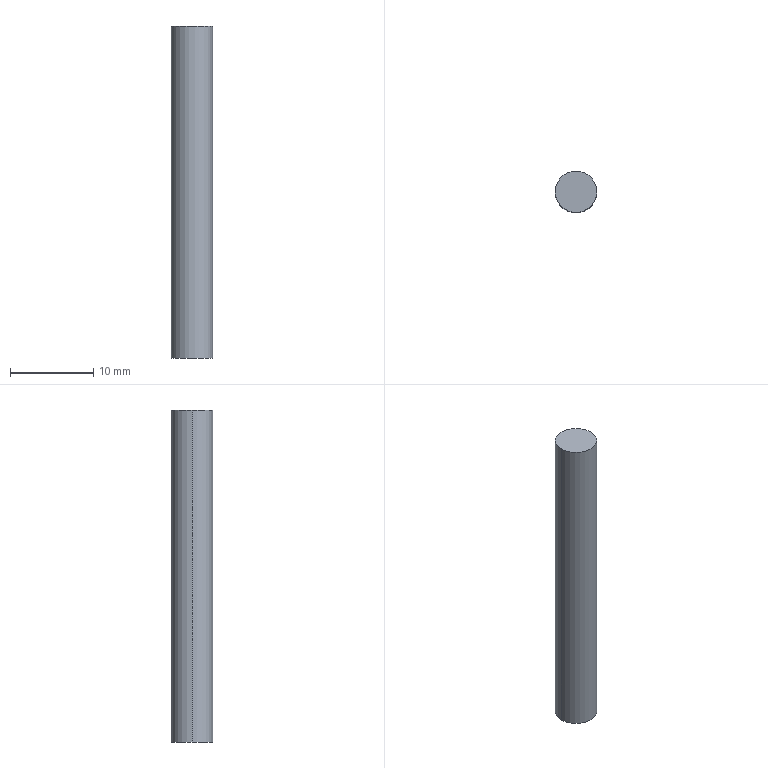Part | SolidWorks | features Extrusion 1 | 1 solid | 4 faces | box 5 x 5 x 40 mm | volume 785.398 mm3 | cylinder 2 | plane 2 | commonest cylinder face diameters 5 x2
STEP:
#1=CARTESIAN_POINT('',(2.5,0.,40.));
#2=VERTEX_POINT('',#1);
#3=CARTESIAN_POINT('',(-2.5,0.,40.));
#4=VERTEX_POINT('',#3);
#5=CARTESIAN_POINT('',(0.,0.,40.));
#6=DIRECTION('',(0.,0.,1.));
#7=DIRECTION('',(1.,0.,0.));
#8=AXIS2_PLACEMENT_3D('',#5,#6,#7);
#9=CIRCLE('',#8,2.5);
#10=EDGE_CURVE('',#2,#4,#9,.T.);
#11=ORIENTED_EDGE('',*,*,#10,.F.);
#12=CARTESIAN_POINT('',(2.5,0.,0.));
#13=VERTEX_POINT('',#12);
#14=CARTESIAN_POINT('',(2.5,0.,40.));
#15=DIRECTION('',(0.,0.,-1.));
#16=VECTOR('',#15,1000.);
#17=LINE('',#14,#16);
#18=EDGE_CURVE('',#2,#13,#17,.T.);
#19=ORIENTED_EDGE('',*,*,#18,.T.);
#20=CARTESIAN_POINT('',(-2.5,0.,0.));
#21=VERTEX_POINT('',#20);
#22=CARTESIAN_POINT('',(0.,0.,0.));
#23=DIRECTION('',(0.,0.,1.));
#24=DIRECTION('',(1.,0.,0.));
#25=AXIS2_PLACEMENT_3D('',#22,#23,#24);
#26=CIRCLE('',#25,2.5);
#27=EDGE_CURVE('',#13,#21,#26,.T.);
#28=ORIENTED_EDGE('',*,*,#27,.T.);
#29=CARTESIAN_POINT('',(-2.5,0.,40.));
#30=DIRECTION('',(0.,0.,-1.));
#31=VECTOR('',#30,1000.);
#32=LINE('',#29,#31);
#33=EDGE_CURVE('',#4,#21,#32,.T.);
#34=ORIENTED_EDGE('',*,*,#33,.F.);
#35=EDGE_LOOP('',(#11,#19,#28,#34));
#36=FACE_OUTER_BOUND('',#35,.T.);
#37=CARTESIAN_POINT('',(0.,0.,40.));
#38=DIRECTION('',(0.,0.,-1.));
#39=DIRECTION('',(-1.,0.,0.));
#40=AXIS2_PLACEMENT_3D('',#37,#38,#39);
#41=CYLINDRICAL_SURFACE('',#40,2.5);
#42=ADVANCED_FACE('',(#36),#41,.T.);
#43=ORIENTED_EDGE('',*,*,#18,.F.);
#44=CARTESIAN_POINT('',(0.,0.,40.));
#45=DIRECTION('',(0.,0.,1.));
#46=DIRECTION('',(1.,0.,0.));
#47=AXIS2_PLACEMENT_3D('',#44,#45,#46);
#48=CIRCLE('',#47,2.5);
#49=EDGE_CURVE('',#4,#2,#48,.T.);
#50=ORIENTED_EDGE('',*,*,#49,.F.);
#51=ORIENTED_EDGE('',*,*,#33,.T.);
#52=CARTESIAN_POINT('',(0.,0.,0.));
#53=DIRECTION('',(0.,0.,1.));
#54=DIRECTION('',(1.,0.,0.));
#55=AXIS2_PLACEMENT_3D('',#52,#53,#54);
#56=CIRCLE('',#55,2.5);
#57=EDGE_CURVE('',#21,#13,#56,.T.);
#58=ORIENTED_EDGE('',*,*,#57,.T.);
#59=EDGE_LOOP('',(#43,#50,#51,#58));
#60=FACE_OUTER_BOUND('',#59,.T.);
#61=CARTESIAN_POINT('',(0.,0.,40.));
#62=DIRECTION('',(0.,0.,-1.));
#63=DIRECTION('',(-1.,0.,0.));
#64=AXIS2_PLACEMENT_3D('',#61,#62,#63);
#65=CYLINDRICAL_SURFACE('',#64,2.5);
#66=ADVANCED_FACE('',(#60),#65,.T.);
#67=ORIENTED_EDGE('',*,*,#49,.T.);
#68=ORIENTED_EDGE('',*,*,#10,.T.);
#69=EDGE_LOOP('',(#67,#68));
#70=FACE_OUTER_BOUND('',#69,.T.);
#71=CARTESIAN_POINT('',(0.,0.,40.));
#72=DIRECTION('',(0.,0.,1.));
#73=DIRECTION('',(1.,0.,0.));
#74=AXIS2_PLACEMENT_3D('',#71,#72,#73);
#75=PLANE('',#74);
#76=ADVANCED_FACE('',(#70),#75,.T.);
#77=ORIENTED_EDGE('',*,*,#57,.F.);
#78=ORIENTED_EDGE('',*,*,#27,.F.);
#79=EDGE_LOOP('',(#77,#78));
#80=FACE_OUTER_BOUND('',#79,.T.);
#81=CARTESIAN_POINT('',(0.,0.,0.));
#82=DIRECTION('',(0.,0.,1.));
#83=DIRECTION('',(1.,0.,0.));
#84=AXIS2_PLACEMENT_3D('',#81,#82,#83);
#85=PLANE('',#84);
#86=ADVANCED_FACE('',(#80),#85,.F.);
#87=CLOSED_SHELL('',(#42,#66,#76,#86));
#88=MANIFOLD_SOLID_BREP('',#87);
#89=CARTESIAN_POINT('',(0.,0.,0.));
#90=DIRECTION('',(0.,0.,1.));
#91=DIRECTION('',(1.,0.,0.));
#92=AXIS2_PLACEMENT_3D('',#89,#90,#91);
#93=(LENGTH_UNIT()NAMED_UNIT(*)SI_UNIT(.MILLI.,.METRE.));
#94=UNCERTAINTY_MEASURE_WITH_UNIT(LENGTH_MEASURE(0.00001),#93,'','');
#95=(NAMED_UNIT(*)PLANE_ANGLE_UNIT()SI_UNIT($,.RADIAN.));
#96=(NAMED_UNIT(*)SI_UNIT($,.STERADIAN.)SOLID_ANGLE_UNIT());
#97=(GEOMETRIC_REPRESENTATION_CONTEXT(3)GLOBAL_UNCERTAINTY_ASSIGNED_CONTEXT((#94))GLOBAL_UNIT_ASSIGNED_CONTEXT((#93,#95,#96))REPRESENTATION_CONTEXT('',''));
#98=ADVANCED_BREP_SHAPE_REPRESENTATION('',(#88,#92),#97);